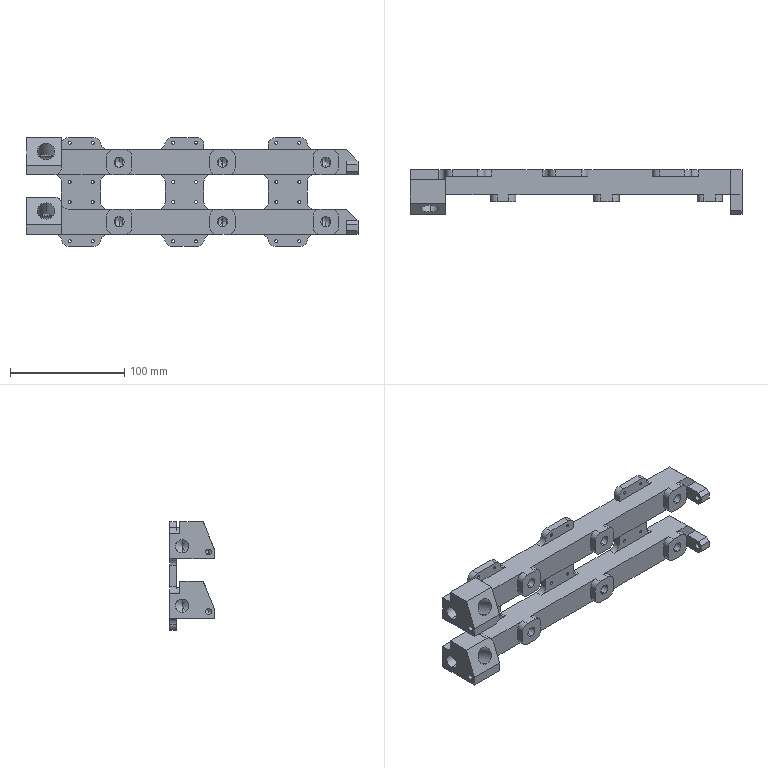Part | 1 solid | 263 faces | box 290 x 39.082 x 95 mm | volume 292360 mm3 | cylinder 155 | plane 82 | cone 26 | commonest cylinder face diameters 12 x61 2.5 x48 8.8 x30 5 x8 11.8 x4 15.25 x4